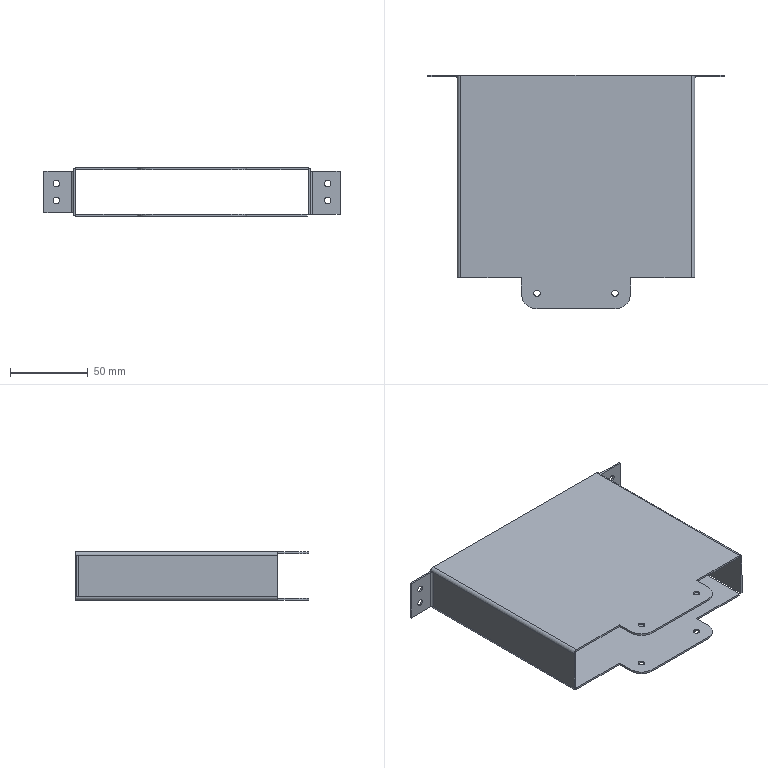Part | SolidWorks | features EdgeFlange 4, Cut 3, Fillet 1, FlatPattern 1, MirrorPattern 1, SMBaseFlange 1, SheetMetal 1 | 1 solid | 77 faces | box 190 x 150 x 31.2 mm | volume 60149 mm3 | plane 47 | cylinder 30 | commonest cylinder face diameters 4.2 x16 2 x5 4.4 x5 20 x4